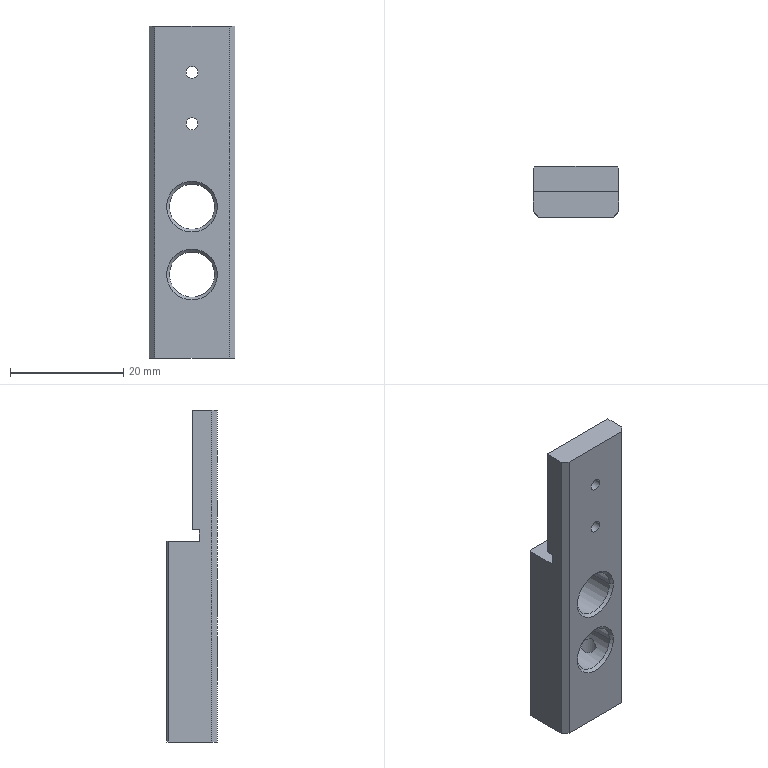Part | NX | 1 solid | 45 faces | box 15.2 x 9 x 58.7 mm | volume 5177 mm3 | cone 19 | plane 14 | cylinder 12 | commonest cylinder face diameters 2.1 x4 3.3 x4 8 x4